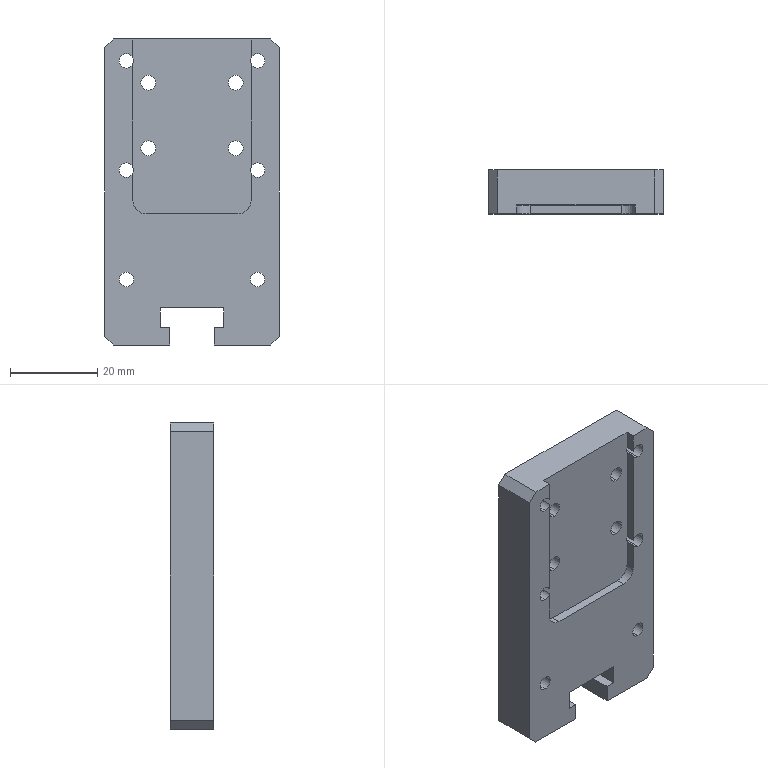Part | STEP file | PN_0016 Mount electronic clip connecting block | 1 solid | 60 faces | box 40 x 10 x 70 mm | volume 23648 mm3 | cylinder 30 | plane 30 | commonest cylinder face diameters 3.3 x12 6 x10 3.4 x8